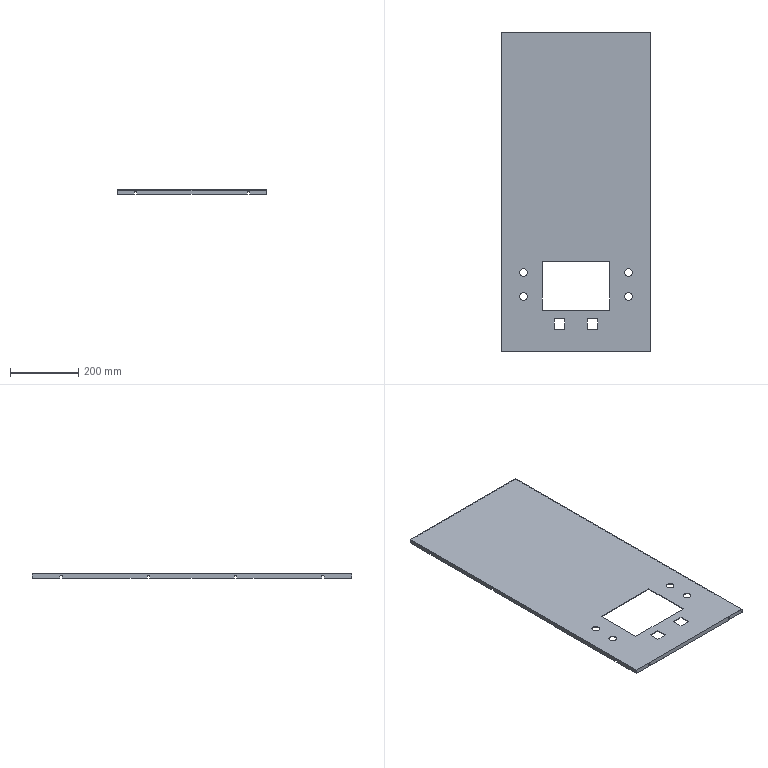Part | SolidWorks | features BaseBody 1 | 1 solid | 82 faces | box 437 x 935 x 12 mm | volume 807325 mm3 | plane 58 | cylinder 24 | commonest cylinder face diameters 7 x16 22.5 x8